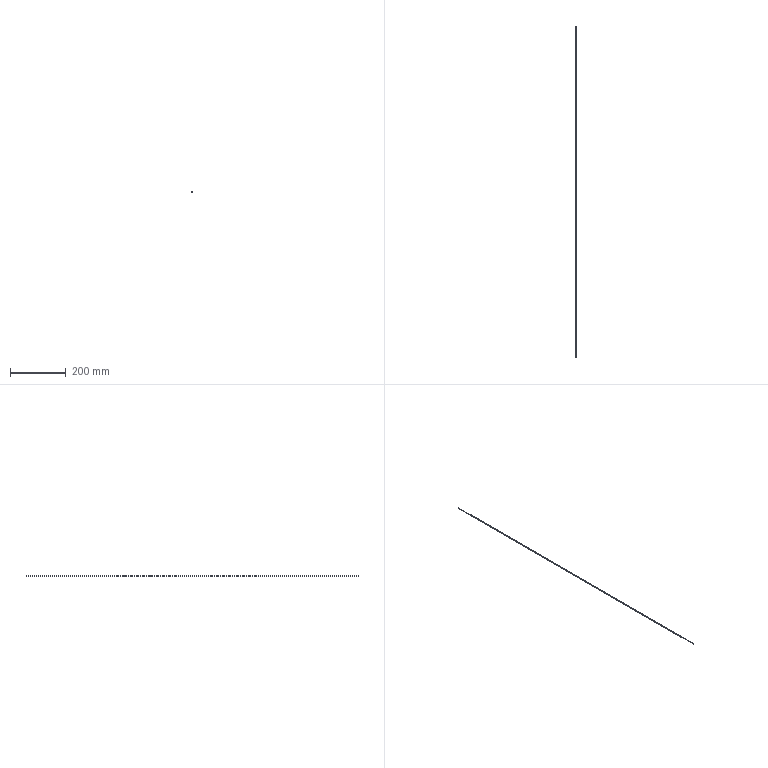Part | NX | features BREP 1 | 1 solid | 6 faces | box 3.5 x 1190 x 0.5 mm | volume 2082 mm3 | plane 6
STEP:
#1=CARTESIAN_POINT('',(1.75,-595.,0.25));
#2=VERTEX_POINT('',#1);
#3=CARTESIAN_POINT('',(1.75,-595.,-0.25));
#4=VERTEX_POINT('',#3);
#5=CARTESIAN_POINT('',(1.75,-595.,-0.25));
#6=DIRECTION('',(0.,0.,-1.));
#7=VECTOR('',#6,1000.);
#8=LINE('',#5,#7);
#9=EDGE_CURVE('',#2,#4,#8,.T.);
#10=ORIENTED_EDGE('',*,*,#9,.F.);
#11=CARTESIAN_POINT('',(-1.75,-595.,0.25));
#12=VERTEX_POINT('',#11);
#13=CARTESIAN_POINT('',(-1.75,-595.,0.25));
#14=DIRECTION('',(1.,0.,0.));
#15=VECTOR('',#14,1000.);
#16=LINE('',#13,#15);
#17=EDGE_CURVE('',#12,#2,#16,.T.);
#18=ORIENTED_EDGE('',*,*,#17,.F.);
#19=CARTESIAN_POINT('',(-1.75,-595.,-0.25));
#20=VERTEX_POINT('',#19);
#21=CARTESIAN_POINT('',(-1.75,-595.,-0.25));
#22=DIRECTION('',(0.,0.,1.));
#23=VECTOR('',#22,1000.);
#24=LINE('',#21,#23);
#25=EDGE_CURVE('',#20,#12,#24,.T.);
#26=ORIENTED_EDGE('',*,*,#25,.F.);
#27=CARTESIAN_POINT('',(-1.75,-595.,-0.25));
#28=DIRECTION('',(-1.,0.,0.));
#29=VECTOR('',#28,1000.);
#30=LINE('',#27,#29);
#31=EDGE_CURVE('',#4,#20,#30,.T.);
#32=ORIENTED_EDGE('',*,*,#31,.F.);
#33=EDGE_LOOP('',(#10,#18,#26,#32));
#34=FACE_BOUND('',#33,.T.);
#35=CARTESIAN_POINT('',(0.,-595.,0.));
#36=DIRECTION('',(0.,1.,0.));
#37=DIRECTION('',(0.,0.,1.));
#38=AXIS2_PLACEMENT_3D('',#35,#36,#37);
#39=PLANE('',#38);
#40=ADVANCED_FACE('',(#34),#39,.F.);
#41=CARTESIAN_POINT('',(1.75,595.,0.25));
#42=VERTEX_POINT('',#41);
#43=CARTESIAN_POINT('',(1.75,595.,-0.25));
#44=VERTEX_POINT('',#43);
#45=CARTESIAN_POINT('',(1.75,595.,-0.25));
#46=DIRECTION('',(0.,0.,-1.));
#47=VECTOR('',#46,1000.);
#48=LINE('',#45,#47);
#49=EDGE_CURVE('',#42,#44,#48,.T.);
#50=ORIENTED_EDGE('',*,*,#49,.T.);
#51=CARTESIAN_POINT('',(-1.75,595.,-0.25));
#52=VERTEX_POINT('',#51);
#53=CARTESIAN_POINT('',(-1.75,595.,-0.25));
#54=DIRECTION('',(-1.,0.,0.));
#55=VECTOR('',#54,1000.);
#56=LINE('',#53,#55);
#57=EDGE_CURVE('',#44,#52,#56,.T.);
#58=ORIENTED_EDGE('',*,*,#57,.T.);
#59=CARTESIAN_POINT('',(-1.75,595.,0.25));
#60=VERTEX_POINT('',#59);
#61=CARTESIAN_POINT('',(-1.75,595.,-0.25));
#62=DIRECTION('',(0.,0.,1.));
#63=VECTOR('',#62,1000.);
#64=LINE('',#61,#63);
#65=EDGE_CURVE('',#52,#60,#64,.T.);
#66=ORIENTED_EDGE('',*,*,#65,.T.);
#67=CARTESIAN_POINT('',(-1.75,595.,0.25));
#68=DIRECTION('',(1.,0.,0.));
#69=VECTOR('',#68,1000.);
#70=LINE('',#67,#69);
#71=EDGE_CURVE('',#60,#42,#70,.T.);
#72=ORIENTED_EDGE('',*,*,#71,.T.);
#73=EDGE_LOOP('',(#50,#58,#66,#72));
#74=FACE_BOUND('',#73,.T.);
#75=CARTESIAN_POINT('',(0.,595.,0.));
#76=DIRECTION('',(0.,1.,0.));
#77=DIRECTION('',(0.,0.,1.));
#78=AXIS2_PLACEMENT_3D('',#75,#76,#77);
#79=PLANE('',#78);
#80=ADVANCED_FACE('',(#74),#79,.T.);
#81=ORIENTED_EDGE('',*,*,#17,.T.);
#82=CARTESIAN_POINT('',(1.75,595.,0.25));
#83=DIRECTION('',(0.,-1.,0.));
#84=VECTOR('',#83,1000.);
#85=LINE('',#82,#84);
#86=EDGE_CURVE('',#42,#2,#85,.T.);
#87=ORIENTED_EDGE('',*,*,#86,.F.);
#88=ORIENTED_EDGE('',*,*,#71,.F.);
#89=CARTESIAN_POINT('',(-1.75,595.,0.25));
#90=DIRECTION('',(0.,-1.,0.));
#91=VECTOR('',#90,1000.);
#92=LINE('',#89,#91);
#93=EDGE_CURVE('',#60,#12,#92,.T.);
#94=ORIENTED_EDGE('',*,*,#93,.T.);
#95=EDGE_LOOP('',(#81,#87,#88,#94));
#96=FACE_BOUND('',#95,.T.);
#97=CARTESIAN_POINT('',(-1.75,595.,0.25));
#98=DIRECTION('',(0.,0.,-1.));
#99=DIRECTION('',(-1.,0.,0.));
#100=AXIS2_PLACEMENT_3D('',#97,#98,#99);
#101=PLANE('',#100);
#102=ADVANCED_FACE('',(#96),#101,.F.);
#103=ORIENTED_EDGE('',*,*,#25,.T.);
#104=ORIENTED_EDGE('',*,*,#93,.F.);
#105=ORIENTED_EDGE('',*,*,#65,.F.);
#106=CARTESIAN_POINT('',(-1.75,595.,-0.25));
#107=DIRECTION('',(0.,-1.,0.));
#108=VECTOR('',#107,1000.);
#109=LINE('',#106,#108);
#110=EDGE_CURVE('',#52,#20,#109,.T.);
#111=ORIENTED_EDGE('',*,*,#110,.T.);
#112=EDGE_LOOP('',(#103,#104,#105,#111));
#113=FACE_BOUND('',#112,.T.);
#114=CARTESIAN_POINT('',(-1.75,595.,-0.25));
#115=DIRECTION('',(1.,0.,0.));
#116=DIRECTION('',(0.,0.,-1.));
#117=AXIS2_PLACEMENT_3D('',#114,#115,#116);
#118=PLANE('',#117);
#119=ADVANCED_FACE('',(#113),#118,.F.);
#120=ORIENTED_EDGE('',*,*,#31,.T.);
#121=ORIENTED_EDGE('',*,*,#110,.F.);
#122=ORIENTED_EDGE('',*,*,#57,.F.);
#123=CARTESIAN_POINT('',(1.75,595.,-0.25));
#124=DIRECTION('',(0.,-1.,0.));
#125=VECTOR('',#124,1000.);
#126=LINE('',#123,#125);
#127=EDGE_CURVE('',#44,#4,#126,.T.);
#128=ORIENTED_EDGE('',*,*,#127,.T.);
#129=EDGE_LOOP('',(#120,#121,#122,#128));
#130=FACE_BOUND('',#129,.T.);
#131=CARTESIAN_POINT('',(-1.75,595.,-0.25));
#132=DIRECTION('',(0.,0.,1.));
#133=DIRECTION('',(1.,0.,0.));
#134=AXIS2_PLACEMENT_3D('',#131,#132,#133);
#135=PLANE('',#134);
#136=ADVANCED_FACE('',(#130),#135,.F.);
#137=ORIENTED_EDGE('',*,*,#9,.T.);
#138=ORIENTED_EDGE('',*,*,#127,.F.);
#139=ORIENTED_EDGE('',*,*,#49,.F.);
#140=ORIENTED_EDGE('',*,*,#86,.T.);
#141=EDGE_LOOP('',(#137,#138,#139,#140));
#142=FACE_BOUND('',#141,.T.);
#143=CARTESIAN_POINT('',(1.75,595.,-0.25));
#144=DIRECTION('',(-1.,0.,0.));
#145=DIRECTION('',(0.,0.,1.));
#146=AXIS2_PLACEMENT_3D('',#143,#144,#145);
#147=PLANE('',#146);
#148=ADVANCED_FACE('',(#142),#147,.F.);
#149=CLOSED_SHELL('',(#40,#80,#102,#119,#136,#148));
#150=MANIFOLD_SOLID_BREP('',#149);
#151=(LENGTH_UNIT()NAMED_UNIT(*)SI_UNIT(.MILLI.,.METRE.));
#152=UNCERTAINTY_MEASURE_WITH_UNIT(LENGTH_MEASURE(0.00001),#151,'','');
#153=(NAMED_UNIT(*)PLANE_ANGLE_UNIT()SI_UNIT($,.RADIAN.));
#154=(NAMED_UNIT(*)SI_UNIT($,.STERADIAN.)SOLID_ANGLE_UNIT());
#155=(GEOMETRIC_REPRESENTATION_CONTEXT(3)GLOBAL_UNCERTAINTY_ASSIGNED_CONTEXT((#152))GLOBAL_UNIT_ASSIGNED_CONTEXT((#151,#153,#154))REPRESENTATION_CONTEXT('',''));
#156=ADVANCED_BREP_SHAPE_REPRESENTATION('',(#150),#155);